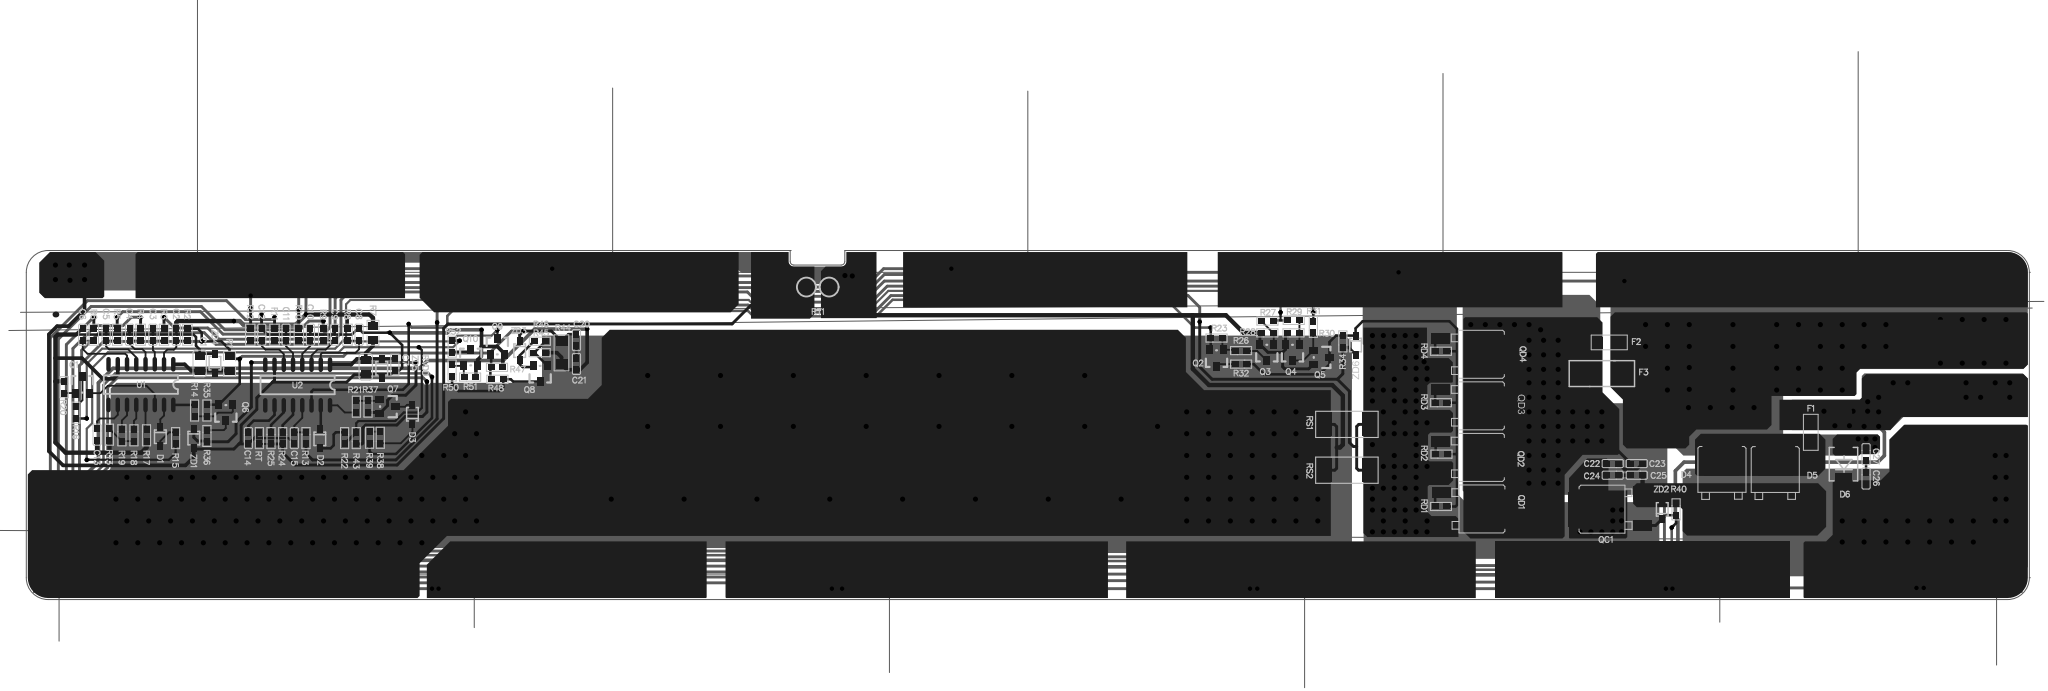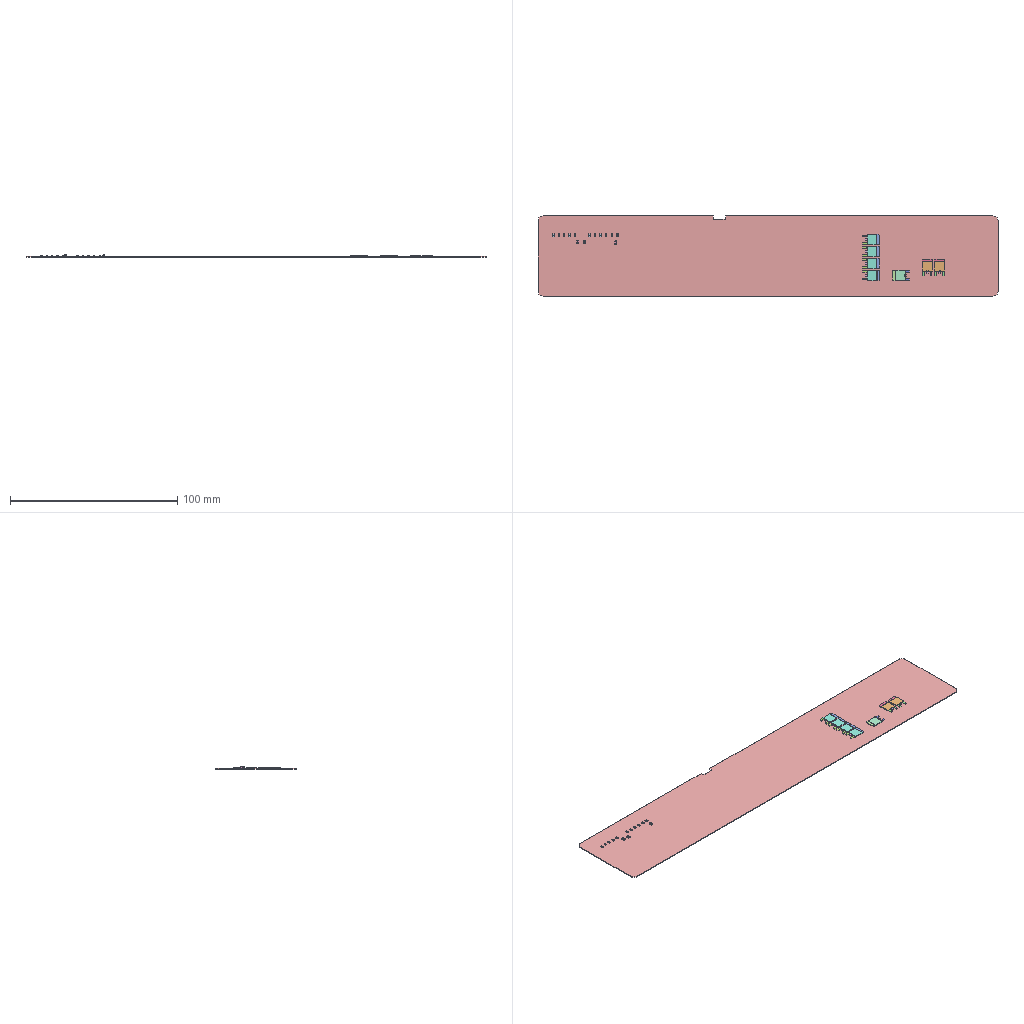Circuit board layout | Altium Designer | box 275 x 48 x 1.3 mm
Layer stack:
# Altium Designer layer stack of  (unit mm; dielectric type: 0 none, 1 core, 2 prepreg, 3 surface material)
index,name,kind,layer,copper_thickness_mm,dielectric_type,dielectric_thickness_mm,dielectric_material,dielectric_constant
0,Top Paste,other,,,,,,
1,Top Overlay,other,,,,,,
2,Top Solder,dielectric,,,3,0.0102,Solder Resist,3.5
3,Top Layer,copper,Top Layer,0.0356,,,,
4,Dielectric 1,dielectric,,,0,0.32,FR-4,4.8
5,Bottom Layer,copper,Bottom Layer,0.0356,,,,
6,Bottom Solder,dielectric,,,3,0.0102,Solder Resist,3.5
7,Bottom Overlay,other,,,,,,
8,Bottom Paste,other,,,,,,
# drill layer pairs: low layer,high layer
drill_pair,Top Layer,Bottom Layer
Part placement:
Designator,Comment,Layer,Footprint,Center-X(mm),Center-Y(mm),Rotation
ZD6,15V,TopLayer,SOD323,182.5,-13,90
QD3,NMOS,TopLayer,TO-252-A,197.883,-21.376,270
R40,3M,TopLayer,R0603A,226.5,-35.6,0
D6,RS2M,TopLayer,SMB-1,249.483,-29.379,90
D5,SS510,TopLayer,TO-252-A,240.129,-32.004,0
R50,1M,TopLayer,R0603A,58.455,-16.505,180
R38,1M,TopLayer,R0603A,48.6,-25.75,180
R36,2M,TopLayer,R0603A,24.8,-25.5,0
R34,5.1M,TopLayer,R0603A,180.75,-12.5,180
F3,NC,TopLayer,2410,216.297,-16.925,0
D2,1N4148,TopLayer,SOD323,40.3,-25.902,90
F2,30A,TopLayer,R1206,217.322,-12.65,0
F1,5A,TopLayer,R1206,245,-25,90
Q3,MMBT5551,TopLayer,SOT-23-3,170.31,-14.01,180
R22,100K,TopLayer,R0603A,43.7,-25.8,0
U2,CW1053,TopLayer,SO-16,37.255,-18.498,180
U1,CW1053,TopLayer,SO-16,15.735,-18.439,180
ZD3,15V,TopLayer,SOD323,67.735,-13.773,90
ZD2,15V,TopLayer,SOD323,224.6,-35.6,270
RVDD,5.1M,TopLayer,R0603A,50.6,-15.7,180
RT,10K,TopLayer,R0603A,32,-25.8,180
RS2,NC,TopLayer,2512,181.317,-30.21,90
RS1,R0015,TopLayer,2512,181.317,-23.91,90
R37,1M,TopLayer,R0603A,46.916,-21.473,0
RT1,103AT,TopLayer,WK,108.662,-5.025,180
R35,1M,TopLayer,R0603A,24.8,-22,180
R32,1K,TopLayer,R0603A,166.78,-15.626,270
R31,2M,TopLayer,R0603A,176.7,-10.5,180
R30,1M,TopLayer,R0603A,173.98,-11.326,90
R29,1M,TopLayer,R0603A,174.007,-9.614,90
R28,1M,TopLayer,R0603A,170.38,-11.326,90
R27,1M,TopLayer,R0603A,170.4,-9.7,90
R26,1M,TopLayer,R0603A,166.772,-13.764,90
R25,35K,TopLayer,R0603A,33.6,-25.8,0
R23,2M,TopLayer,R0603A,163.409,-12.039,90
R21,5.1M,TopLayer,R0603A,45.316,-21.473,180
R20,2M,TopLayer,R0603A,5.2,-18.8,0
R19,35K,TopLayer,R0603A,13.13,-25.416,0
R18,22K,TopLayer,R0603A,14.78,-25.416,0
R17,1K,TopLayer,R0603A,16.505,-25.416,0
R16,5.1M,TopLayer,R0603A,6.8,-22.3,180
R15,51K,TopLayer,R0603A,20.5,-25.8,0
R14,5.1M,TopLayer,R0603A,23.1,-22,0
R13,1K,TopLayer,R0603A,38.4,-25.8,0
R11,1K,TopLayer,RES0603,34.084,-11.581,180
R10,1K,TopLayer,RES0603,37.423,-11.581,0
R12,1K,TopLayer,RES0603,30.746,-11.581,0
R9,1K,TopLayer,RES0603,40.761,-11.581,0
R8,1K,TopLayer,RES0603,44.099,-11.581,0
R7,1K,TopLayer,RES0805,47.6,-11.329,270
R6,1K,TopLayer,RES0603,9.268,-11.581,0
R5,1K,TopLayer,RES0603,12.481,-11.581,0
R4,1K,TopLayer,RES0603,15.693,-11.581,0
R3,1K,TopLayer,RES0603,18.906,-11.581,0
R2,1K,TopLayer,RES0603,22.119,-11.581,0
R1,1K,TopLayer,RES0805,27.9,-15.584,270
QD4,NMOS,TopLayer,TO-252-A,197.883,-14.287,270
QD2,NMOS,TopLayer,TO-252-A,197.883,-28.466,270
QC1,NMOS,TopLayer,TO-252-A,218.215,-35.555,90
Q5,MMBT5551,TopLayer,SOT-23-3,177.8,-14.7,270
Q4,MMBT5551,TopLayer,SOT-23-3,173.836,-14.01,180
Q2,BSS84,TopLayer,SOT-23-3,163.409,-14.767,180
D4,SS510,TopLayer,TO-252-A,232.815,-31.985,0
D3,1N4148,TopLayer,SOD323,53.016,-22.516,270
D1,1N4148,TopLayer,SOD323,18.4,-25.608,90
C15,0.1uF,TopLayer,C0603A,36.8,-25.8,180
C14,0.1uF,TopLayer,C0603A,30.5,-25.8,0
C13,0.1uF,TopLayer,C0603A,9.718,-25.324,0
C12,0.1uF,TopLayer,C0603A,32.327,-11.58,180
C11,0.1uF,TopLayer,C0603A,35.665,-11.58,180
C10,0.1uF,TopLayer,C0603A,39.003,-11.58,180
C9,0.1uF,TopLayer,C0603A,42.341,-11.58,180
C8,0.1uF,TopLayer,C0603A,45.68,-11.58,180
C7,1uF,TopLayer,CAP0805,46.6,-16.016,270
C6,0.1uF,TopLayer,C0603A,7.75,-11.58,180
C5,0.1uF,TopLayer,C0603A,10.963,-11.58,180
C4,0.1uF,TopLayer,C0603A,14.175,-11.58,180
C3,0.1uF,TopLayer,C0603A,17.388,-11.58,180
C2,0.1uF,TopLayer,C0603A,20.601,-11.58,180
C1,1uF,TopLayer,CAP0805,23.8,-15.517,90
RD2,47R,TopLayer,R0603A,194.292,-28.002,90
C20,0.1uf,TopLayer,C0603A,75.535,-12.323,0
C21,0.1uf,TopLayer,C0603A,75.535,-15.598,0
Q1,MMBT5401,TopLayer,SOT-23-3,7.7,-18.5,0
Q6,MMBT5401,TopLayer,SOT-23-3,27.4,-22.303,180
Q7,MMBT5401,TopLayer,SOT-23-3,49.616,-21.473,270
Q8,MMBT5401,TopLayer,SOT-23-3,70.547,-16.907,180
Q9,MMBT5551,TopLayer,SOT-23-3,64.668,-13.237,0
Q10,MMBT5551,TopLayer,SOT-23-3,61.017,-14.746,0
QD1,NMOS,TopLayer,TO-252-A,197.963,-35.556,270
R39,1M,TopLayer,R0603A,47.125,-25.75,180
R43,100K,TopLayer,R0603A,45.3,-25.8,180
R44,47K/1206,TopLayer,R1206,73.485,-14.073,90
R45,1M,TopLayer,R0603A,70.485,-14.048,90
R46,51K,TopLayer,R0603A,70.51,-12.473,90
R47,100K,TopLayer,R0603A,64.622,-16.065,90
R48,1M,TopLayer,R0603A,64.68,-17.703,90
R51,100K,TopLayer,R0603A,60.93,-17.405,90
R52,1K,TopLayer,R0603A,58.467,-13.226,0
RD1,47R,TopLayer,R0603A,194.217,-35.202,90
RD3,47R,TopLayer,R0603A,194.217,-20.927,90
RD4,47R,TopLayer,R0603A,194.217,-13.852,90
RT3,10K,TopLayer,R0603A,11.418,-25.324,0
ZD1,24V,TopLayer,SOD323,23,-25.8,90
R24,22K,TopLayer,R0603A,35.2,-25.8,0
C22,0.1uF,TopLayer,C0603A,217.8,-29.3,270
C23,0.1uF,TopLayer,C0603A,221.1,-29.3,90
C24,0.1uF,TopLayer,C0603A,217.8,-30.9,270
C25,0.1uF,TopLayer,C0603A,221.1,-30.9,270
C26,0.1uF,TopLayer,C0603A,252.583,-31.354,0
C27,0.1uF,TopLayer,C0603A,252.583,-28.016,0
ZD4,24V,TopLayer,SOD323,25.9,-15.5,270
ZD5,24V,TopLayer,SOD323,48.8,-16.2,90
Pad and via stacks:
# Altium Designer via and pad stacks of  (unit mm). Each distinct definition once, with the count of objects using it.
# via: kind,start_layer,end_layer,hole_mm,diameter_mm,mode(0 simple;1 top-mid-bottom;2 full stack),diameter_per_layer,count,example_net
# pad: kind,layer,hole_mm,hole_type(0 round;1 square;2 slot),plating,top_size,top_shape(1 round;2 rect;3 octagon;9 rounded rect),mid_size,bottom_size,mode,footprint,size_per_layer,count,example
pad,Top Layer,0,0,plated,1.27x1.1,2,1.27x1.1,1.27x1.1,0,CAP0805,,2,C7.1
pad,Top Layer,0,0,plated,1.27x1.016,2,1.27x1.016,1.27x1.016,0,CAP0805,,2,C7.2
pad,Top Layer,0,0,plated,0.9x0.8,2,0.9x0.8,0.9x0.8,0,C0603A,,21,C15.1
pad,Top Layer,0,0,unplated,0.9x0.8,2,0.9x0.8,0.9x0.8,0,C0603A,,21,C15.2
pad,Top Layer,0,0,plated,1x0.8,2,1x0.8,1x0.8,0,SOD323,,18,D3.1
pad,Top Layer,0,0,plated,1.5x2.5,2,1.5x2.5,1.5x2.5,0,TO-252-A,,7,QD4.1
pad,Top Layer,0,0,plated,4.8x5.5,2,4.8x5.5,4.8x5.5,0,TO-252-A,,7,QD4.3
pad,Top Layer,0,0,plated,1.8x2.5,2,1.8x2.5,1.8x2.5,0,TO-252-A,,7,QD4.2
pad,Top Layer,0,0,plated,1.27x1.016,2,1.27x1.016,1.27x1.016,0,RES0805,,4,R7.2
pad,Top Layer,0,0,plated,0.83x0.88,2,0.83x0.88,0.83x0.88,0,RES0603,,20,R11.1
pad,Top Layer,0,0,plated,2.2x2.2,1,2.2x2.2,2.2x2.2,0,WK,,2,RT1.1
pad,Top Layer,0,0,plated,2x3.2,2,2x3.2,2x3.2,0,2512,,4,RS2.2
pad,Top Layer,0,0,plated,2.032x0.6096,1,2.032x0.6096,2.032x0.6096,0,SO-16,,32,U2.10
pad,Top Layer,0,0,plated,0.9144x1.2,2,0.9144x1.2,0.9144x1.2,0,SOT-23-3,,30,Q3.3
pad,Top Layer,0,0,plated,1.3x1.6,2,1.3x1.6,1.3x1.6,0,R1206,,6,F2.2
pad,Top Layer,0,0,plated,2.8x3.15,2,2.8x3.15,2.8x3.15,0,2410,,2,F3.2
pad,Top Layer,0,0,unplated,0.9x0.8,2,0.9x0.8,0.9x0.8,0,R0603A,,42,R50.2
pad,Top Layer,0,0,plated,0.9x0.8,2,0.9x0.8,0.9x0.8,0,R0603A,,42,R50.1
pad,Top Layer,0,0,plated,1.8x2.3,2,1.8x2.3,1.8x2.3,0,SMB-1,,2,D6.1
pad,Top Layer,0,2,plated,0.8x0.8,1,0.8x0.8,0.8x0.8,0,,,3,600
pad,Top Layer,0,0,plated,2.5x2.5,1,2.5x2.5,2.5x2.5,0,,,15,1
pad,Top Layer,0,0,plated,1x1,1,1x1,1x1,0,,,1,1
pad,Top Layer,0,0,plated,8x5,2,8x5,8x5,0,,,11,12
pad,Top Layer,0,0,plated,5x3,1,5x3,5x3,0,,,2,16
pad,Top Layer,0,0,plated,9x5,1,9x5,9x5,0,,,2,14
via,Top Layer,Bottom Layer,0.5,0.7,0,,362,P-
via,Top Layer,Bottom Layer,0.4,0.6,0,,48,VM
Copper pours:
name,layer,net,type(0 solid;1 hatched;2 none)
Top Layer-P- 2,Top Layer,P-,0
Top Layer-NetC25_1,Top Layer,NetC25_1,0
Top Layer-NetD4_2,Top Layer,NetD4_3,0
NONET_L-01_P-001,Top Layer,B7,0
Top Layer-CS,Top Layer,CS,0
Top Layer-NetC23_1,Top Layer,NetC23_1,0
b,Top Layer,CS,0
Top Layer-B- 1,Top Layer,B-,0
Top Layer-B+,Top Layer,B+,0
NONET_L-01_P-001,Top Layer,B9,0
NONET_L-01_P-001,Top Layer,B3,0
NONET_L-01_P-001,Top Layer,NetR24_2,0
Top Layer-P- 1,Top Layer,P-,0
NONET_L-01_P-001,Top Layer,B5,0
Top Layer-P-,Top Layer,P-,0
Top Layer-C-,Top Layer,C-,0
NONET_L-01_P-001,Top Layer,B1,0
Top Layer-B-,Top Layer,B-,0
NONET_L-01_P-001,Top Layer,B-,0
NONET_L-01_P-001,Top Layer,B8,0
NONET_L-01_P-001,Top Layer,B6,0
NONET_L-01_P-001,Top Layer,B4,0
NONET_L-01_P-001,Top Layer,B2,0
Bottom Layer-CS,Bottom Layer,CS,0
Bottom Layer-NetC23_1,Bottom Layer,NetC23_1,0
Bottom Layer-B- 1,Bottom Layer,B-,0
Bottom Layer-B+,Bottom Layer,B+,0
Bottom Layer-P-,Bottom Layer,P-,0
Bottom Layer-B-,Bottom Layer,B-,0
Bottom Layer-C-,Bottom Layer,C-,0
Bottom Layer-P- 1,Bottom Layer,P-,0
Design rules, without the lines most boards share:
# Altium Designer design rules of  (exported by Altium Designer, unit mm)
# columns: name | kind | enabled | priority | scope1 | scope2 | descriptor | typed fields (field=value)
Stitching CS | 0 | enabled | 1 | IsStitchingVia and InNet('CS') | (IsVia and (Not IsStitchingVia)) Or IsPad | Clearance Constraint (Gap=0.127mm) (IsStitchingVia and InNet('CS')),((IsVia and (Not IsStitchingVia)) Or IsPad) | gap=0.127
NetAntennae | 56 | enabled | 1 | All | All | Net Antennae (Tolerance=0mm) (All) |
SilkToSilkClearance | 55 | enabled | 1 | All | All | Silk to Silk (Clearance=0.254mm) (All),(All) |
SilkToSolderMaskClearance | 54 | enabled | 1 | IsPad | All | Silk To Solder Mask (Clearance=0.254mm) (IsPad),(All) |
MinimumSolderMaskSliver | 53 | enabled | 1 | All | All | Minimum Solder Mask Sliver (Gap=0.254mm) (All),(All) |
HoleToHoleClearance | 52 | enabled | 1 | All | All | Hole To Hole Clearance (Gap=0.254mm) (All),(All) | gap=0.254
DiffPairsRouting | 51 | enabled | 1 | All | All | Differential Pairs Uncoupled Length using the Gap Constraints (Min=0.254mm) (Max=0.254mm) (Prefered=0.254mm)  and Width Constraints (Min=0.381mm) (Max=0.381mm) (Prefered=0.381mm) (All) |
HoleSize | 42 | enabled | 1 | All | All | Hole Size Constraint (Min=0.025mm) (Max=2.54mm) (All) |
Height | 50 | enabled | 1 | All | All | Height Constraint (Min=0mm) (Max=25.4mm) (Prefered=12.7mm) (All) | min_height=0 max_height=25.4
ComponentClearance | 24 | enabled | 1 | All | All | Component Clearance Constraint ( Horizontal Gap = 0.2mm, Vertical Gap = 0.254mm ) (All),(All)  | gap=0.2
SolderMaskExpansion | 13 | enabled | 1 | All | All | Solder Mask Expansion (Expansion =0.102mm) (All) | expansion=0.1016
PasteMaskExpansion | 14 | enabled | 1 | All | All | Paste Mask Expansion (Expansion =0mm) (All) | expansion=0
RoutingVias | 11 | enabled | 1 | All | All | Routing Via (MinHoleWidth=0.4mm) (MaxHoleWidth=0.4mm) (PreferredHoleWidth=0.4mm) (MinWidth=0.6mm) (MaxWidth=0.6mm) (PreferedWidth=0.6mm) (All) | via_min_hole=0.4 via_max_hole=0.4 via_preferred_diameter=0.6 via_preferred_hole=0.4
RoutingCorners | 10 | enabled | 1 | All | All | Routing Corners (Style=45-Degree) (Min Setback=2.54mm) (Max Setback=2.54mm) (All) |
Width | 2 | enabled | 1 | All | All | Width Constraint (Min=0.2mm) (Max=1mm) (Preferred=0.25mm) (All) |
PolygonConnect | 20 | enabled | 1 | All | All | Polygon Connect Rule(Direct Connect )(Conductor Width=0.254mm) (Relief Angle=90 Angle) (Entries=4) (Air Gap Width=0.254mm) (All),(All) | connect_style(0=relief,1=direct,2=none)=1 relief_conductor_width=0.254 relief_entries=4
PlaneClearance | 12 | enabled | 1 | All | All | Power Plane Clearance (Clearance =0.508mm) (All) | clearance=0.508
PlaneConnect | 6 | enabled | 1 | All | All | Power Plane Connect Rule(Relief Connect )(Expansion=0.508mm) (Conductor Width=0.254mm) (Air Gap=0.254mm) (Entries=4) (All) | relief_conductor_width=0.254 relief_entries=4 relief_expansion=0.508
Clearance | 0 | enabled | 2 | All | All | Clearance Constraint (Gap=0.2mm) (All),(All) | gap=0.2